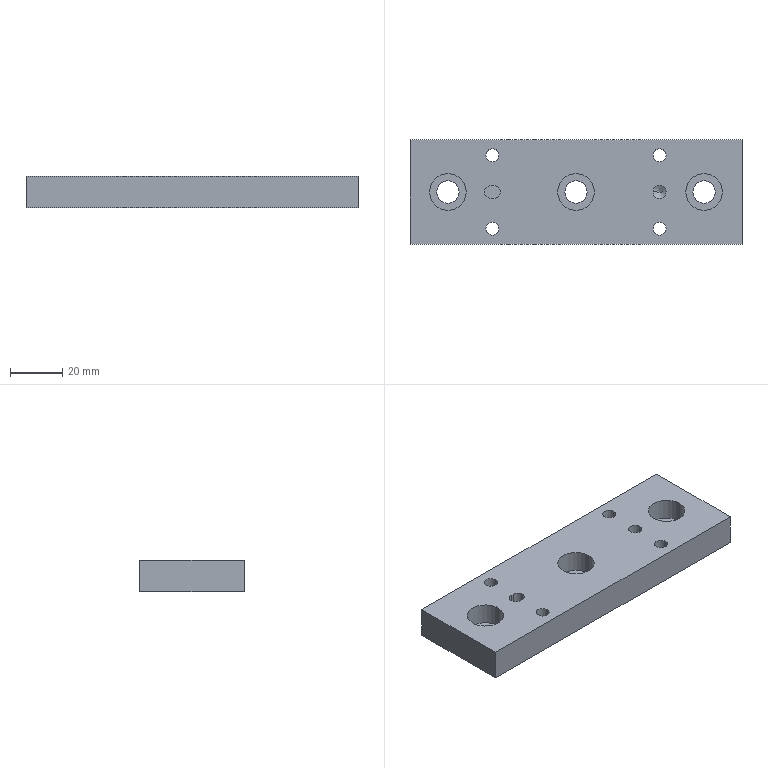Part | STEP file | 1 solid | 42 faces | box 127 x 40 x 12 mm | volume 55019 mm3 | cylinder 27 | plane 13 | cone 2 | commonest cylinder face diameters 5 x13 8.5 x6 14 x6 29.1 x2
STEP:
#1=CARTESIAN_POINT('',(14.55,0.,0.5));
#2=VERTEX_POINT('',#1);
#3=CARTESIAN_POINT('',(-14.55,0.,0.5));
#4=VERTEX_POINT('',#3);
#5=CARTESIAN_POINT('',(0.,0.,0.5));
#6=DIRECTION('',(0.,0.,-1.));
#7=DIRECTION('',(-1.,0.,0.));
#8=AXIS2_PLACEMENT_3D('',#5,#6,#7);
#9=CIRCLE('',#8,14.55);
#10=EDGE_CURVE('',#2,#4,#9,.T.);
#11=ORIENTED_EDGE('',*,*,#10,.F.);
#12=CARTESIAN_POINT('',(14.55,0.,0.));
#13=VERTEX_POINT('',#12);
#14=CARTESIAN_POINT('',(14.55,0.,0.5));
#15=DIRECTION('',(0.,0.,-1.));
#16=VECTOR('',#15,1000.);
#17=LINE('',#14,#16);
#18=EDGE_CURVE('',#2,#13,#17,.T.);
#19=ORIENTED_EDGE('',*,*,#18,.T.);
#20=CARTESIAN_POINT('',(-14.55,0.,0.));
#21=VERTEX_POINT('',#20);
#22=CARTESIAN_POINT('',(0.,0.,0.));
#23=DIRECTION('',(0.,0.,-1.));
#24=DIRECTION('',(-1.,0.,0.));
#25=AXIS2_PLACEMENT_3D('',#22,#23,#24);
#26=CIRCLE('',#25,14.55);
#27=EDGE_CURVE('',#13,#21,#26,.T.);
#28=ORIENTED_EDGE('',*,*,#27,.T.);
#29=CARTESIAN_POINT('',(-14.55,0.,0.5));
#30=DIRECTION('',(0.,0.,-1.));
#31=VECTOR('',#30,1000.);
#32=LINE('',#29,#31);
#33=EDGE_CURVE('',#4,#21,#32,.T.);
#34=ORIENTED_EDGE('',*,*,#33,.F.);
#35=EDGE_LOOP('',(#11,#19,#28,#34));
#36=FACE_OUTER_BOUND('',#35,.T.);
#37=CARTESIAN_POINT('',(0.,0.,0.5));
#38=DIRECTION('',(0.,0.,-1.));
#39=DIRECTION('',(-1.,0.,0.));
#40=AXIS2_PLACEMENT_3D('',#37,#38,#39);
#41=CYLINDRICAL_SURFACE('',#40,14.55);
#42=ADVANCED_FACE('',(#36),#41,.F.);
#43=CARTESIAN_POINT('',(42.,0.,3.7));
#44=VERTEX_POINT('',#43);
#45=CARTESIAN_POINT('',(56.,0.,3.7));
#46=VERTEX_POINT('',#45);
#47=CARTESIAN_POINT('',(49.,0.,3.7));
#48=DIRECTION('',(0.,0.,1.));
#49=DIRECTION('',(1.,0.,0.));
#50=AXIS2_PLACEMENT_3D('',#47,#48,#49);
#51=CIRCLE('',#50,7.);
#52=EDGE_CURVE('',#44,#46,#51,.T.);
#53=ORIENTED_EDGE('',*,*,#52,.F.);
#54=CARTESIAN_POINT('',(42.,0.,12.));
#55=VERTEX_POINT('',#54);
#56=CARTESIAN_POINT('',(42.,0.,12.));
#57=DIRECTION('',(0.,0.,1.));
#58=VECTOR('',#57,1000.);
#59=LINE('',#56,#58);
#60=EDGE_CURVE('',#44,#55,#59,.T.);
#61=ORIENTED_EDGE('',*,*,#60,.T.);
#62=CARTESIAN_POINT('',(56.,0.,12.));
#63=VERTEX_POINT('',#62);
#64=CARTESIAN_POINT('',(49.,0.,12.));
#65=DIRECTION('',(0.,0.,1.));
#66=DIRECTION('',(1.,0.,0.));
#67=AXIS2_PLACEMENT_3D('',#64,#65,#66);
#68=CIRCLE('',#67,7.);
#69=EDGE_CURVE('',#55,#63,#68,.T.);
#70=ORIENTED_EDGE('',*,*,#69,.T.);
#71=CARTESIAN_POINT('',(56.,0.,12.));
#72=DIRECTION('',(0.,0.,1.));
#73=VECTOR('',#72,1000.);
#74=LINE('',#71,#73);
#75=EDGE_CURVE('',#46,#63,#74,.T.);
#76=ORIENTED_EDGE('',*,*,#75,.F.);
#77=EDGE_LOOP('',(#53,#61,#70,#76));
#78=FACE_OUTER_BOUND('',#77,.T.);
#79=CARTESIAN_POINT('',(49.,0.,12.));
#80=DIRECTION('',(0.,0.,1.));
#81=DIRECTION('',(1.,0.,0.));
#82=AXIS2_PLACEMENT_3D('',#79,#80,#81);
#83=CYLINDRICAL_SURFACE('',#82,7.);
#84=ADVANCED_FACE('',(#78),#83,.F.);
#85=CARTESIAN_POINT('',(44.75,0.,0.));
#86=VERTEX_POINT('',#85);
#87=CARTESIAN_POINT('',(53.25,0.,0.));
#88=VERTEX_POINT('',#87);
#89=CARTESIAN_POINT('',(49.,0.,0.));
#90=DIRECTION('',(0.,0.,1.));
#91=DIRECTION('',(1.,0.,0.));
#92=AXIS2_PLACEMENT_3D('',#89,#90,#91);
#93=CIRCLE('',#92,4.25);
#94=EDGE_CURVE('',#86,#88,#93,.T.);
#95=ORIENTED_EDGE('',*,*,#94,.F.);
#96=CARTESIAN_POINT('',(44.75,0.,3.7));
#97=VERTEX_POINT('',#96);
#98=CARTESIAN_POINT('',(44.75,0.,12.));
#99=DIRECTION('',(0.,0.,1.));
#100=VECTOR('',#99,1000.);
#101=LINE('',#98,#100);
#102=EDGE_CURVE('',#86,#97,#101,.T.);
#103=ORIENTED_EDGE('',*,*,#102,.T.);
#104=CARTESIAN_POINT('',(53.25,0.,3.7));
#105=VERTEX_POINT('',#104);
#106=CARTESIAN_POINT('',(49.,0.,3.7));
#107=DIRECTION('',(0.,0.,1.));
#108=DIRECTION('',(1.,0.,0.));
#109=AXIS2_PLACEMENT_3D('',#106,#107,#108);
#110=CIRCLE('',#109,4.25);
#111=EDGE_CURVE('',#97,#105,#110,.T.);
#112=ORIENTED_EDGE('',*,*,#111,.T.);
#113=CARTESIAN_POINT('',(53.25,0.,12.));
#114=DIRECTION('',(0.,0.,1.));
#115=VECTOR('',#114,1000.);
#116=LINE('',#113,#115);
#117=EDGE_CURVE('',#88,#105,#116,.T.);
#118=ORIENTED_EDGE('',*,*,#117,.F.);
#119=EDGE_LOOP('',(#95,#103,#112,#118));
#120=FACE_OUTER_BOUND('',#119,.T.);
#121=CARTESIAN_POINT('',(49.,0.,12.));
#122=DIRECTION('',(0.,0.,1.));
#123=DIRECTION('',(1.,0.,0.));
#124=AXIS2_PLACEMENT_3D('',#121,#122,#123);
#125=CYLINDRICAL_SURFACE('',#124,4.25);
#126=ADVANCED_FACE('',(#120),#125,.F.);
#127=CARTESIAN_POINT('',(-56.,0.,3.7));
#128=VERTEX_POINT('',#127);
#129=CARTESIAN_POINT('',(-42.,0.,3.7));
#130=VERTEX_POINT('',#129);
#131=CARTESIAN_POINT('',(-49.,0.,3.7));
#132=DIRECTION('',(0.,0.,1.));
#133=DIRECTION('',(1.,0.,0.));
#134=AXIS2_PLACEMENT_3D('',#131,#132,#133);
#135=CIRCLE('',#134,7.);
#136=EDGE_CURVE('',#128,#130,#135,.T.);
#137=ORIENTED_EDGE('',*,*,#136,.F.);
#138=CARTESIAN_POINT('',(-56.,0.,12.));
#139=VERTEX_POINT('',#138);
#140=CARTESIAN_POINT('',(-56.,0.,12.));
#141=DIRECTION('',(0.,0.,1.));
#142=VECTOR('',#141,1000.);
#143=LINE('',#140,#142);
#144=EDGE_CURVE('',#128,#139,#143,.T.);
#145=ORIENTED_EDGE('',*,*,#144,.T.);
#146=CARTESIAN_POINT('',(-42.,0.,12.));
#147=VERTEX_POINT('',#146);
#148=CARTESIAN_POINT('',(-49.,0.,12.));
#149=DIRECTION('',(0.,0.,1.));
#150=DIRECTION('',(1.,0.,0.));
#151=AXIS2_PLACEMENT_3D('',#148,#149,#150);
#152=CIRCLE('',#151,7.);
#153=EDGE_CURVE('',#139,#147,#152,.T.);
#154=ORIENTED_EDGE('',*,*,#153,.T.);
#155=CARTESIAN_POINT('',(-42.,0.,12.));
#156=DIRECTION('',(0.,0.,1.));
#157=VECTOR('',#156,1000.);
#158=LINE('',#155,#157);
#159=EDGE_CURVE('',#130,#147,#158,.T.);
#160=ORIENTED_EDGE('',*,*,#159,.F.);
#161=EDGE_LOOP('',(#137,#145,#154,#160));
#162=FACE_OUTER_BOUND('',#161,.T.);
#163=CARTESIAN_POINT('',(-49.,0.,12.));
#164=DIRECTION('',(0.,0.,1.));
#165=DIRECTION('',(1.,0.,0.));
#166=AXIS2_PLACEMENT_3D('',#163,#164,#165);
#167=CYLINDRICAL_SURFACE('',#166,7.);
#168=ADVANCED_FACE('',(#162),#167,.F.);
#169=CARTESIAN_POINT('',(-53.25,0.,0.));
#170=VERTEX_POINT('',#169);
#171=CARTESIAN_POINT('',(-44.75,0.,0.));
#172=VERTEX_POINT('',#171);
#173=CARTESIAN_POINT('',(-49.,0.,0.));
#174=DIRECTION('',(0.,0.,1.));
#175=DIRECTION('',(1.,0.,0.));
#176=AXIS2_PLACEMENT_3D('',#173,#174,#175);
#177=CIRCLE('',#176,4.25);
#178=EDGE_CURVE('',#170,#172,#177,.T.);
#179=ORIENTED_EDGE('',*,*,#178,.F.);
#180=CARTESIAN_POINT('',(-53.25,0.,3.7));
#181=VERTEX_POINT('',#180);
#182=CARTESIAN_POINT('',(-53.25,0.,12.));
#183=DIRECTION('',(0.,0.,1.));
#184=VECTOR('',#183,1000.);
#185=LINE('',#182,#184);
#186=EDGE_CURVE('',#170,#181,#185,.T.);
#187=ORIENTED_EDGE('',*,*,#186,.T.);
#188=CARTESIAN_POINT('',(-44.75,0.,3.7));
#189=VERTEX_POINT('',#188);
#190=CARTESIAN_POINT('',(-49.,0.,3.7));
#191=DIRECTION('',(0.,0.,1.));
#192=DIRECTION('',(1.,0.,0.));
#193=AXIS2_PLACEMENT_3D('',#190,#191,#192);
#194=CIRCLE('',#193,4.25);
#195=EDGE_CURVE('',#181,#189,#194,.T.);
#196=ORIENTED_EDGE('',*,*,#195,.T.);
#197=CARTESIAN_POINT('',(-44.75,0.,12.));
#198=DIRECTION('',(0.,0.,1.));
#199=VECTOR('',#198,1000.);
#200=LINE('',#197,#199);
#201=EDGE_CURVE('',#172,#189,#200,.T.);
#202=ORIENTED_EDGE('',*,*,#201,.F.);
#203=EDGE_LOOP('',(#179,#187,#196,#202));
#204=FACE_OUTER_BOUND('',#203,.T.);
#205=CARTESIAN_POINT('',(-49.,0.,12.));
#206=DIRECTION('',(0.,0.,1.));
#207=DIRECTION('',(1.,0.,0.));
#208=AXIS2_PLACEMENT_3D('',#205,#206,#207);
#209=CYLINDRICAL_SURFACE('',#208,4.25);
#210=ADVANCED_FACE('',(#204),#209,.F.);
#211=CARTESIAN_POINT('',(29.5,14.,0.));
#212=VERTEX_POINT('',#211);
#213=CARTESIAN_POINT('',(34.5,14.,0.));
#214=VERTEX_POINT('',#213);
#215=CARTESIAN_POINT('',(32.,14.,0.));
#216=DIRECTION('',(0.,0.,1.));
#217=DIRECTION('',(1.,0.,0.));
#218=AXIS2_PLACEMENT_3D('',#215,#216,#217);
#219=CIRCLE('',#218,2.5);
#220=EDGE_CURVE('',#212,#214,#219,.T.);
#221=ORIENTED_EDGE('',*,*,#220,.F.);
#222=CARTESIAN_POINT('',(29.5,14.,12.));
#223=VERTEX_POINT('',#222);
#224=CARTESIAN_POINT('',(29.5,14.,12.));
#225=DIRECTION('',(0.,0.,1.));
#226=VECTOR('',#225,1000.);
#227=LINE('',#224,#226);
#228=EDGE_CURVE('',#212,#223,#227,.T.);
#229=ORIENTED_EDGE('',*,*,#228,.T.);
#230=CARTESIAN_POINT('',(34.5,14.,12.));
#231=VERTEX_POINT('',#230);
#232=CARTESIAN_POINT('',(32.,14.,12.));
#233=DIRECTION('',(0.,0.,1.));
#234=DIRECTION('',(1.,0.,0.));
#235=AXIS2_PLACEMENT_3D('',#232,#233,#234);
#236=CIRCLE('',#235,2.5);
#237=EDGE_CURVE('',#223,#231,#236,.T.);
#238=ORIENTED_EDGE('',*,*,#237,.T.);
#239=CARTESIAN_POINT('',(34.5,14.,12.));
#240=DIRECTION('',(0.,0.,1.));
#241=VECTOR('',#240,1000.);
#242=LINE('',#239,#241);
#243=EDGE_CURVE('',#214,#231,#242,.T.);
#244=ORIENTED_EDGE('',*,*,#243,.F.);
#245=EDGE_LOOP('',(#221,#229,#238,#244));
#246=FACE_OUTER_BOUND('',#245,.T.);
#247=CARTESIAN_POINT('',(32.,14.,12.));
#248=DIRECTION('',(0.,0.,1.));
#249=DIRECTION('',(1.,0.,0.));
#250=AXIS2_PLACEMENT_3D('',#247,#248,#249);
#251=CYLINDRICAL_SURFACE('',#250,2.5);
#252=ADVANCED_FACE('',(#246),#251,.F.);
#253=CARTESIAN_POINT('',(29.5,-14.,0.));
#254=VERTEX_POINT('',#253);
#255=CARTESIAN_POINT('',(34.5,-14.,0.));
#256=VERTEX_POINT('',#255);
#257=CARTESIAN_POINT('',(32.,-14.,0.));
#258=DIRECTION('',(0.,0.,1.));
#259=DIRECTION('',(1.,0.,0.));
#260=AXIS2_PLACEMENT_3D('',#257,#258,#259);
#261=CIRCLE('',#260,2.5);
#262=EDGE_CURVE('',#254,#256,#261,.T.);
#263=ORIENTED_EDGE('',*,*,#262,.F.);
#264=CARTESIAN_POINT('',(29.5,-14.,12.));
#265=VERTEX_POINT('',#264);
#266=CARTESIAN_POINT('',(29.5,-14.,12.));
#267=DIRECTION('',(0.,0.,1.));
#268=VECTOR('',#267,1000.);
#269=LINE('',#266,#268);
#270=EDGE_CURVE('',#254,#265,#269,.T.);
#271=ORIENTED_EDGE('',*,*,#270,.T.);
#272=CARTESIAN_POINT('',(34.5,-14.,12.));
#273=VERTEX_POINT('',#272);
#274=CARTESIAN_POINT('',(32.,-14.,12.));
#275=DIRECTION('',(0.,0.,1.));
#276=DIRECTION('',(1.,0.,0.));
#277=AXIS2_PLACEMENT_3D('',#274,#275,#276);
#278=CIRCLE('',#277,2.5);
#279=EDGE_CURVE('',#265,#273,#278,.T.);
#280=ORIENTED_EDGE('',*,*,#279,.T.);
#281=CARTESIAN_POINT('',(34.5,-14.,12.));
#282=DIRECTION('',(0.,0.,1.));
#283=VECTOR('',#282,1000.);
#284=LINE('',#281,#283);
#285=EDGE_CURVE('',#256,#273,#284,.T.);
#286=ORIENTED_EDGE('',*,*,#285,.F.);
#287=EDGE_LOOP('',(#263,#271,#280,#286));
#288=FACE_OUTER_BOUND('',#287,.T.);
#289=CARTESIAN_POINT('',(32.,-14.,12.));
#290=DIRECTION('',(0.,0.,1.));
#291=DIRECTION('',(1.,0.,0.));
#292=AXIS2_PLACEMENT_3D('',#289,#290,#291);
#293=CYLINDRICAL_SURFACE('',#292,2.5);
#294=ADVANCED_FACE('',(#288),#293,.F.);
#295=CARTESIAN_POINT('',(-34.5,-14.,0.));
#296=VERTEX_POINT('',#295);
#297=CARTESIAN_POINT('',(-29.5,-14.,0.));
#298=VERTEX_POINT('',#297);
#299=CARTESIAN_POINT('',(-32.,-14.,0.));
#300=DIRECTION('',(0.,0.,1.));
#301=DIRECTION('',(1.,0.,0.));
#302=AXIS2_PLACEMENT_3D('',#299,#300,#301);
#303=CIRCLE('',#302,2.5);
#304=EDGE_CURVE('',#296,#298,#303,.T.);
#305=ORIENTED_EDGE('',*,*,#304,.F.);
#306=CARTESIAN_POINT('',(-34.5,-14.,12.));
#307=VERTEX_POINT('',#306);
#308=CARTESIAN_POINT('',(-34.5,-14.,12.));
#309=DIRECTION('',(0.,0.,1.));
#310=VECTOR('',#309,1000.);
#311=LINE('',#308,#310);
#312=EDGE_CURVE('',#296,#307,#311,.T.);
#313=ORIENTED_EDGE('',*,*,#312,.T.);
#314=CARTESIAN_POINT('',(-29.5,-14.,12.));
#315=VERTEX_POINT('',#314);
#316=CARTESIAN_POINT('',(-32.,-14.,12.));
#317=DIRECTION('',(0.,0.,1.));
#318=DIRECTION('',(1.,0.,0.));
#319=AXIS2_PLACEMENT_3D('',#316,#317,#318);
#320=CIRCLE('',#319,2.5);
#321=EDGE_CURVE('',#307,#315,#320,.T.);
#322=ORIENTED_EDGE('',*,*,#321,.T.);
#323=CARTESIAN_POINT('',(-29.5,-14.,12.));
#324=DIRECTION('',(0.,0.,1.));
#325=VECTOR('',#324,1000.);
#326=LINE('',#323,#325);
#327=EDGE_CURVE('',#298,#315,#326,.T.);
#328=ORIENTED_EDGE('',*,*,#327,.F.);
#329=EDGE_LOOP('',(#305,#313,#322,#328));
#330=FACE_OUTER_BOUND('',#329,.T.);
#331=CARTESIAN_POINT('',(-32.,-14.,12.));
#332=DIRECTION('',(0.,0.,1.));
#333=DIRECTION('',(1.,0.,0.));
#334=AXIS2_PLACEMENT_3D('',#331,#332,#333);
#335=CYLINDRICAL_SURFACE('',#334,2.5);
#336=ADVANCED_FACE('',(#330),#335,.F.);
#337=CARTESIAN_POINT('',(-34.5,14.,0.));
#338=VERTEX_POINT('',#337);
#339=CARTESIAN_POINT('',(-29.5,14.,0.));
#340=VERTEX_POINT('',#339);
#341=CARTESIAN_POINT('',(-32.,14.,0.));
#342=DIRECTION('',(0.,0.,1.));
#343=DIRECTION('',(1.,0.,0.));
#344=AXIS2_PLACEMENT_3D('',#341,#342,#343);
#345=CIRCLE('',#344,2.5);
#346=EDGE_CURVE('',#338,#340,#345,.T.);
#347=ORIENTED_EDGE('',*,*,#346,.F.);
#348=CARTESIAN_POINT('',(-34.5,14.,12.));
#349=VERTEX_POINT('',#348);
#350=CARTESIAN_POINT('',(-34.5,14.,12.));
#351=DIRECTION('',(0.,0.,1.));
#352=VECTOR('',#351,1000.);
#353=LINE('',#350,#352);
#354=EDGE_CURVE('',#338,#349,#353,.T.);
#355=ORIENTED_EDGE('',*,*,#354,.T.);
#356=CARTESIAN_POINT('',(-29.5,14.,12.));
#357=VERTEX_POINT('',#356);
#358=CARTESIAN_POINT('',(-32.,14.,12.));
#359=DIRECTION('',(0.,0.,1.));
#360=DIRECTION('',(1.,0.,0.));
#361=AXIS2_PLACEMENT_3D('',#358,#359,#360);
#362=CIRCLE('',#361,2.5);
#363=EDGE_CURVE('',#349,#357,#362,.T.);
#364=ORIENTED_EDGE('',*,*,#363,.T.);
#365=CARTESIAN_POINT('',(-29.5,14.,12.));
#366=DIRECTION('',(0.,0.,1.));
#367=VECTOR('',#366,1000.);
#368=LINE('',#365,#367);
#369=EDGE_CURVE('',#340,#357,#368,.T.);
#370=ORIENTED_EDGE('',*,*,#369,.F.);
#371=EDGE_LOOP('',(#347,#355,#364,#370));
#372=FACE_OUTER_BOUND('',#371,.T.);
#373=CARTESIAN_POINT('',(-32.,14.,12.));
#374=DIRECTION('',(0.,0.,1.));
#375=DIRECTION('',(1.,0.,0.));
#376=AXIS2_PLACEMENT_3D('',#373,#374,#375);
#377=CYLINDRICAL_SURFACE('',#376,2.5);
#378=ADVANCED_FACE('',(#372),#377,.F.);
#379=CARTESIAN_POINT('',(-7.,0.,3.7));
#380=VERTEX_POINT('',#379);
#381=CARTESIAN_POINT('',(7.,0.,3.7));
#382=VERTEX_POINT('',#381);
#383=CARTESIAN_POINT('',(0.,0.,3.7));
#384=DIRECTION('',(0.,0.,1.));
#385=DIRECTION('',(1.,0.,0.));
#386=AXIS2_PLACEMENT_3D('',#383,#384,#385);
#387=CIRCLE('',#386,7.);
#388=EDGE_CURVE('',#380,#382,#387,.T.);
#389=ORIENTED_EDGE('',*,*,#388,.F.);
#390=CARTESIAN_POINT('',(-7.,0.,12.));
#391=VERTEX_POINT('',#390);
#392=CARTESIAN_POINT('',(-7.,0.,12.));
#393=DIRECTION('',(0.,0.,1.));
#394=VECTOR('',#393,1000.);
#395=LINE('',#392,#394);
#396=EDGE_CURVE('',#380,#391,#395,.T.);
#397=ORIENTED_EDGE('',*,*,#396,.T.);
#398=CARTESIAN_POINT('',(7.,0.,12.));
#399=VERTEX_POINT('',#398);
#400=CARTESIAN_POINT('',(0.,0.,12.));
#401=DIRECTION('',(0.,0.,1.));
#402=DIRECTION('',(1.,0.,0.));
#403=AXIS2_PLACEMENT_3D('',#400,#401,#402);
#404=CIRCLE('',#403,7.);
#405=EDGE_CURVE('',#391,#399,#404,.T.);
#406=ORIENTED_EDGE('',*,*,#405,.T.);
#407=CARTESIAN_POINT('',(7.,0.,12.));
#408=DIRECTION('',(0.,0.,1.));
#409=VECTOR('',#408,1000.);
#410=LINE('',#407,#409);
#411=EDGE_CURVE('',#382,#399,#410,.T.);
#412=ORIENTED_EDGE('',*,*,#411,.F.);
#413=EDGE_LOOP('',(#389,#397,#406,#412));
#414=FACE_OUTER_BOUND('',#413,.T.);
#415=CARTESIAN_POINT('',(0.,0.,12.));
#416=DIRECTION('',(0.,0.,1.));
#417=DIRECTION('',(1.,0.,0.));
#418=AXIS2_PLACEMENT_3D('',#415,#416,#417);
#419=CYLINDRICAL_SURFACE('',#418,7.);
#420=ADVANCED_FACE('',(#414),#419,.F.);
#421=CARTESIAN_POINT('',(-29.,0.,7.));
#422=VERTEX_POINT('',#421);
#423=CARTESIAN_POINT('',(-31.5,2.5,7.));
#424=VERTEX_POINT('',#423);
#425=CARTESIAN_POINT('',(-31.5,0.,7.));
#426=DIRECTION('',(0.,0.,1.));
#427=DIRECTION('',(1.,0.,0.));
#428=AXIS2_PLACEMENT_3D('',#425,#426,#427);
#429=CIRCLE('',#428,2.5);
#430=EDGE_CURVE('',#422,#424,#429,.T.);
#431=ORIENTED_EDGE('',*,*,#430,.F.);
#432=CARTESIAN_POINT('',(-29.,0.,12.));
#433=VERTEX_POINT('',#432);
#434=CARTESIAN_POINT('',(-29.,0.,7.));
#435=DIRECTION('',(0.,0.,1.));
#436=VECTOR('',#435,1000.);
#437=LINE('',#434,#436);
#438=EDGE_CURVE('',#422,#433,#437,.T.);
#439=ORIENTED_EDGE('',*,*,#438,.T.);
#440=CARTESIAN_POINT('',(-31.5,2.5,12.));
#441=VERTEX_POINT('',#440);
#442=CARTESIAN_POINT('',(-31.5,0.,12.));
#443=DIRECTION('',(0.,0.,1.));
#444=DIRECTION('',(1.,0.,0.));
#445=AXIS2_PLACEMENT_3D('',#442,#443,#444);
#446=CIRCLE('',#445,2.5);
#447=EDGE_CURVE('',#433,#441,#446,.T.);
#448=ORIENTED_EDGE('',*,*,#447,.T.);
#449=CARTESIAN_POINT('',(-31.5,2.5,7.));
#450=DIRECTION('',(0.,0.,1.));
#451=VECTOR('',#450,1000.);
#452=LINE('',#449,#451);
#453=EDGE_CURVE('',#424,#441,#452,.T.);
#454=ORIENTED_EDGE('',*,*,#453,.F.);
#455=EDGE_LOOP('',(#431,#439,#448,#454));
#456=FACE_OUTER_BOUND('',#455,.T.);
#457=CARTESIAN_POINT('',(-31.5,0.,7.));
#458=DIRECTION('',(0.,0.,1.));
#459=DIRECTION('',(1.,0.,0.));
#460=AXIS2_PLACEMENT_3D('',#457,#458,#459);
#461=CYLINDRICAL_SURFACE('',#460,2.5);
#462=ADVANCED_FACE('',(#456),#461,.F.);
#463=CARTESIAN_POINT('',(29.5,0.,7.));
#464=VERTEX_POINT('',#463);
#465=CARTESIAN_POINT('',(34.5,0.,7.));
#466=VERTEX_POINT('',#465);
#467=CARTESIAN_POINT('',(32.,0.,7.));
#468=DIRECTION('',(0.,0.,1.));
#469=DIRECTION('',(1.,0.,0.));
#470=AXIS2_PLACEMENT_3D('',#467,#468,#469);
#471=CIRCLE('',#470,2.5);
#472=EDGE_CURVE('',#464,#466,#471,.T.);
#473=ORIENTED_EDGE('',*,*,#472,.F.);
#474=CARTESIAN_POINT('',(29.5,0.,12.));
#475=VERTEX_POINT('',#474);
#476=CARTESIAN_POINT('',(29.5,0.,12.));
#477=DIRECTION('',(0.,0.,1.));
#478=VECTOR('',#477,1000.);
#479=LINE('',#476,#478);
#480=EDGE_CURVE('',#464,#475,#479,.T.);
#481=ORIENTED_EDGE('',*,*,#480,.T.);
#482=CARTESIAN_POINT('',(34.5,0.,12.));
#483=VERTEX_POINT('',#482);
#484=CARTESIAN_POINT('',(32.,0.,12.));
#485=DIRECTION('',(0.,0.,1.));
#486=DIRECTION('',(1.,0.,0.));
#487=AXIS2_PLACEMENT_3D('',#484,#485,#486);
#488=CIRCLE('',#487,2.5);
#489=EDGE_CURVE('',#475,#483,#488,.T.);
#490=ORIENTED_EDGE('',*,*,#489,.T.);
#491=CARTESIAN_POINT('',(34.5,0.,12.));
#492=DIRECTION('',(0.,0.,1.));
#493=VECTOR('',#492,1000.);
#494=LINE('',#491,#493);
#495=EDGE_CURVE('',#466,#483,#494,.T.);
#496=ORIENTED_EDGE('',*,*,#495,.F.);
#497=EDGE_LOOP('',(#473,#481,#490,#496));
#498=FACE_OUTER_BOUND('',#497,.T.);
#499=CARTESIAN_POINT('',(32.,0.,12.));
#500=DIRECTION('',(0.,0.,1.));
#501=DIRECTION('',(1.,0.,0.));
#502=AXIS2_PLACEMENT_3D('',#499,#500,#501);
#503=CYLINDRICAL_SURFACE('',#502,2.5);
#504=ADVANCED_FACE('',(#498),#503,.F.);
#505=CARTESIAN_POINT('',(32.,0.,5.498));
#506=VERTEX_POINT('',#505);
#507=CARTESIAN_POINT('',(34.5,0.,7.));
#508=DIRECTION('',(0.8572,0.,0.515));
#509=VECTOR('',#508,1000.);
#510=LINE('',#507,#509);
#511=EDGE_CURVE('',#506,#466,#510,.T.);
#512=ORIENTED_EDGE('',*,*,#511,.F.);
#513=CARTESIAN_POINT('',(29.5,0.,7.));
#514=DIRECTION('',(-0.8572,0.,0.515));
#515=VECTOR('',#514,1000.);
#516=LINE('',#513,#515);
#517=EDGE_CURVE('',#506,#464,#516,.T.);
#518=ORIENTED_EDGE('',*,*,#517,.T.);
#519=ORIENTED_EDGE('',*,*,#472,.T.);
#520=EDGE_LOOP('',(#512,#518,#519));
#521=FACE_OUTER_BOUND('',#520,.T.);
#522=CARTESIAN_POINT('',(32.,0.,7.));
#523=DIRECTION('',(0.,0.,1.));
#524=DIRECTION('',(1.,0.,0.));
#525=AXIS2_PLACEMENT_3D('',#522,#523,#524);
#526=CONICAL_SURFACE('',#525,2.5,1.03);
#527=ADVANCED_FACE('',(#521),#526,.F.);
#528=CARTESIAN_POINT('',(-4.25,0.,0.5));
#529=VERTEX_POINT('',#528);
#530=CARTESIAN_POINT('',(4.25,0.,0.5));
#531=VERTEX_POINT('',#530);
#532=CARTESIAN_POINT('',(0.,0.,0.5));
#533=DIRECTION('',(0.,0.,1.));
#534=DIRECTION('',(-1.,0.,0.));
#535=AXIS2_PLACEMENT_3D('',#532,#533,#534);
#536=CIRCLE('',#535,4.25);
#537=EDGE_CURVE('',#529,#531,#536,.T.);
#538=ORIENTED_EDGE('',*,*,#537,.F.);
#539=CARTESIAN_POINT('',(-4.25,0.,3.7));
#540=VERTEX_POINT('',#539);
#541=CARTESIAN_POINT('',(-4.25,0.,12.));
#542=DIRECTION('',(0.,0.,1.));
#543=VECTOR('',#542,1000.);
#544=LINE('',#541,#543);
#545=EDGE_CURVE('',#529,#540,#544,.T.);
#546=ORIENTED_EDGE('',*,*,#545,.T.);
#547=CARTESIAN_POINT('',(4.25,0.,3.7));
#548=VERTEX_POINT('',#547);
#549=CARTESIAN_POINT('',(0.,0.,3.7));
#550=DIRECTION('',(0.,0.,1.));
#551=DIRECTION('',(1.,0.,0.));
#552=AXIS2_PLACEMENT_3D('',#549,#550,#551);
#553=CIRCLE('',#552,4.25);
#554=EDGE_CURVE('',#540,#548,#553,.T.);
#555=ORIENTED_EDGE('',*,*,#554,.T.);
#556=CARTESIAN_POINT('',(4.25,0.,12.));
#557=DIRECTION('',(0.,0.,1.));
#558=VECTOR('',#557,1000.);
#559=LINE('',#556,#558);
#560=EDGE_CURVE('',#531,#548,#559,.T.);
#561=ORIENTED_EDGE('',*,*,#560,.F.);
#562=EDGE_LOOP('',(#538,#546,#555,#561));
#563=FACE_OUTER_BOUND('',#562,.T.);
#564=CARTESIAN_POINT('',(0.,0.,12.));
#565=DIRECTION('',(0.,0.,1.));
#566=DIRECTION('',(1.,0.,0.));
#567=AXIS2_PLACEMENT_3D('',#564,#565,#566);
#568=CYLINDRICAL_SURFACE('',#567,4.25);
#569=ADVANCED_FACE('',(#563),#568,.F.);
#570=ORIENTED_EDGE('',*,*,#545,.F.);
#571=CARTESIAN_POINT('',(0.,0.,0.5));
#572=DIRECTION('',(0.,0.,1.));
#573=DIRECTION('',(-1.,0.,0.));
#574=AXIS2_PLACEMENT_3D('',#571,#572,#573);
#575=CIRCLE('',#574,4.25);
#576=EDGE_CURVE('',#531,#529,#575,.T.);
#577=ORIENTED_EDGE('',*,*,#576,.F.);
#578=ORIENTED_EDGE('',*,*,#560,.T.);
#579=CARTESIAN_POINT('',(0.,0.,3.7));
#580=DIRECTION('',(0.,0.,1.));
#581=DIRECTION('',(1.,0.,0.));
#582=AXIS2_PLACEMENT_3D('',#579,#580,#581);
#583=CIRCLE('',#582,4.25);
#584=EDGE_CURVE('',#548,#540,#583,.T.);
#585=ORIENTED_EDGE('',*,*,#584,.T.);
#586=EDGE_LOOP('',(#570,#577,#578,#585));
#587=FACE_OUTER_BOUND('',#586,.T.);
#588=CARTESIAN_POINT('',(0.,0.,12.));
#589=DIRECTION('',(0.,0.,1.));
#590=DIRECTION('',(1.,0.,0.));
#591=AXIS2_PLACEMENT_3D('',#588,#589,#590);
#592=CYLINDRICAL_SURFACE('',#591,4.25);
#593=ADVANCED_FACE('',(#587),#592,.F.);
#594=CARTESIAN_POINT('',(63.5,-20.,0.));
#595=VERTEX_POINT('',#594);
#596=CARTESIAN_POINT('',(63.5,20.,0.));
#597=VERTEX_POINT('',#596);
#598=CARTESIAN_POINT('',(63.5,-20.,0.));
#599=DIRECTION('',(0.,1.,0.));
#600=VECTOR('',#599,1000.);
#601=LINE('',#598,#600);
#602=EDGE_CURVE('',#595,#597,#601,.T.);
#603=ORIENTED_EDGE('',*,*,#602,.T.);
#604=CARTESIAN_POINT('',(63.5,20.,12.));
#605=VERTEX_POINT('',#604);
#606=CARTESIAN_POINT('',(63.5,20.,12.));
#607=DIRECTION('',(0.,0.,-1.));
#608=VECTOR('',#607,1000.);
#609=LINE('',#606,#608);
#610=EDGE_CURVE('',#605,#597,#609,.T.);
#611=ORIENTED_EDGE('',*,*,#610,.F.);
#612=CARTESIAN_POINT('',(63.5,-20.,12.));
#613=VERTEX_POINT('',#612);
#614=CARTESIAN_POINT('',(63.5,-20.,12.));
#615=DIRECTION('',(0.,1.,0.));
#616=VECTOR('',#615,1000.);
#617=LINE('',#614,#616);
#618=EDGE_CURVE('',#613,#605,#617,.T.);
#619=ORIENTED_EDGE('',*,*,#618,.F.);
#620=CARTESIAN_POINT('',(63.5,-20.,12.));
#621=DIRECTION('',(0.,0.,-1.));
#622=VECTOR('',#621,1000.);
#623=LINE('',#620,#622);
#624=EDGE_CURVE('',#613,#595,#623,.T.);
#625=ORIENTED_EDGE('',*,*,#624,.T.);
#626=EDGE_LOOP('',(#603,#611,#619,#625));
#627=FACE_OUTER_BOUND('',#626,.T.);
#628=CARTESIAN_POINT('',(63.5,-20.,12.));
#629=DIRECTION('',(-1.,0.,0.));
#630=DIRECTION('',(0.,0.,1.));
#631=AXIS2_PLACEMENT_3D('',#628,#629,#630);
#632=PLANE('',#631);
#633=ADVANCED_FACE('',(#627),#632,.F.);
#634=CARTESIAN_POINT('',(-63.5,20.,0.));
#635=VERTEX_POINT('',#634);
#636=CARTESIAN_POINT('',(-63.5,20.,0.));
#637=DIRECTION('',(-1.,0.,0.));
#638=VECTOR('',#637,1000.);
#639=LINE('',#636,#638);
#640=EDGE_CURVE('',#597,#635,#639,.T.);
#641=ORIENTED_EDGE('',*,*,#640,.T.);
#642=CARTESIAN_POINT('',(-63.5,20.,12.));
#643=VERTEX_POINT('',#642);
#644=CARTESIAN_POINT('',(-63.5,20.,12.));
#645=DIRECTION('',(0.,0.,-1.));
#646=VECTOR('',#645,1000.);
#647=LINE('',#644,#646);
#648=EDGE_CURVE('',#643,#635,#647,.T.);
#649=ORIENTED_EDGE('',*,*,#648,.F.);
#650=CARTESIAN_POINT('',(-63.5,20.,12.));
#651=DIRECTION('',(-1.,0.,0.));
#652=VECTOR('',#651,1000.);
#653=LINE('',#650,#652);
#654=EDGE_CURVE('',#605,#643,#653,.T.);
#655=ORIENTED_EDGE('',*,*,#654,.F.);
#656=ORIENTED_EDGE('',*,*,#610,.T.);
#657=EDGE_LOOP('',(#641,#649,#655,#656));
#658=FACE_OUTER_BOUND('',#657,.T.);
#659=CARTESIAN_POINT('',(-63.5,20.,12.));
#660=DIRECTION('',(0.,-1.,0.));
#661=DIRECTION('',(0.,0.,-1.));
#662=AXIS2_PLACEMENT_3D('',#659,#660,#661);
#663=PLANE('',#662);
#664=ADVANCED_FACE('',(#658),#663,.F.);
#665=CARTESIAN_POINT('',(-63.5,-20.,0.));
#666=VERTEX_POINT('',#665);
#667=CARTESIAN_POINT('',(-63.5,-20.,0.));
#668=DIRECTION('',(0.,-1.,0.));
#669=VECTOR('',#668,1000.);
#670=LINE('',#667,#669);
#671=EDGE_CURVE('',#635,#666,#670,.T.);
#672=ORIENTED_EDGE('',*,*,#671,.T.);
#673=CARTESIAN_POINT('',(-63.5,-20.,12.));
#674=VERTEX_POINT('',#673);
#675=CARTESIAN_POINT('',(-63.5,-20.,12.));
#676=DIRECTION('',(0.,0.,-1.));
#677=VECTOR('',#676,1000.);
#678=LINE('',#675,#677);
#679=EDGE_CURVE('',#674,#666,#678,.T.);
#680=ORIENTED_EDGE('',*,*,#679,.F.);
#681=CARTESIAN_POINT('',(-63.5,-20.,12.));
#682=DIRECTION('',(0.,-1.,0.));
#683=VECTOR('',#682,1000.);
#684=LINE('',#681,#683);
#685=EDGE_CURVE('',#643,#674,#684,.T.);
#686=ORIENTED_EDGE('',*,*,#685,.F.);
#687=ORIENTED_EDGE('',*,*,#648,.T.);
#688=EDGE_LOOP('',(#672,#680,#686,#687));
#689=FACE_OUTER_BOUND('',#688,.T.);
#690=CARTESIAN_POINT('',(-63.5,-20.,12.));
#691=DIRECTION('',(1.,0.,0.));
#692=DIRECTION('',(0.,1.,0.));
#693=AXIS2_PLACEMENT_3D('',#690,#691,#692);
#694=PLANE('',#693);
#695=ADVANCED_FACE('',(#689),#694,.F.);
#696=CARTESIAN_POINT('',(-63.5,-20.,0.));
#697=DIRECTION('',(1.,0.,0.));
#698=VECTOR('',#697,1000.);
#699=LINE('',#696,#698);
#700=EDGE_CURVE('',#666,#595,#699,.T.);
#701=ORIENTED_EDGE('',*,*,#700,.T.);
#702=ORIENTED_EDGE('',*,*,#624,.F.);
#703=CARTESIAN_POINT('',(-63.5,-20.,12.));
#704=DIRECTION('',(1.,0.,0.));
#705=VECTOR('',#704,1000.);
#706=LINE('',#703,#705);
#707=EDGE_CURVE('',#674,#613,#706,.T.);
#708=ORIENTED_EDGE('',*,*,#707,.F.);
#709=ORIENTED_EDGE('',*,*,#679,.T.);
#710=EDGE_LOOP('',(#701,#702,#708,#709));
#711=FACE_OUTER_BOUND('',#710,.T.);
#712=CARTESIAN_POINT('',(-63.5,-20.,12.));
#713=DIRECTION('',(0.,1.,0.));
#714=DIRECTION('',(1.,0.,0.));
#715=AXIS2_PLACEMENT_3D('',#712,#713,#714);
#716=PLANE('',#715);
#717=ADVANCED_FACE('',(#711),#716,.F.);
#718=ORIENTED_EDGE('',*,*,#618,.T.);
#719=ORIENTED_EDGE('',*,*,#654,.T.);
#720=ORIENTED_EDGE('',*,*,#685,.T.);
#721=ORIENTED_EDGE('',*,*,#707,.T.);
#722=EDGE_LOOP('',(#718,#719,#720,#721));
#723=FACE_OUTER_BOUND('',#722,.T.);
#724=CARTESIAN_POINT('',(49.,0.,12.));
#725=DIRECTION('',(0.,0.,1.));
#726=DIRECTION('',(1.,0.,0.));
#727=AXIS2_PLACEMENT_3D('',#724,#725,#726);
#728=CIRCLE('',#727,7.);
#729=EDGE_CURVE('',#63,#55,#728,.T.);
#730=ORIENTED_EDGE('',*,*,#729,.F.);
#731=ORIENTED_EDGE('',*,*,#69,.F.);
#732=EDGE_LOOP('',(#730,#731));
#733=FACE_BOUND('',#732,.T.);
#734=CARTESIAN_POINT('',(-49.,0.,12.));
#735=DIRECTION('',(0.,0.,1.));
#736=DIRECTION('',(1.,0.,0.));
#737=AXIS2_PLACEMENT_3D('',#734,#735,#736);
#738=CIRCLE('',#737,7.);
#739=EDGE_CURVE('',#147,#139,#738,.T.);
#740=ORIENTED_EDGE('',*,*,#739,.F.);
#741=ORIENTED_EDGE('',*,*,#153,.F.);
#742=EDGE_LOOP('',(#740,#741));
#743=FACE_BOUND('',#742,.T.);
#744=CARTESIAN_POINT('',(32.,14.,12.));
#745=DIRECTION('',(0.,0.,1.));
#746=DIRECTION('',(1.,0.,0.));
#747=AXIS2_PLACEMENT_3D('',#744,#745,#746);
#748=CIRCLE('',#747,2.5);
#749=EDGE_CURVE('',#231,#223,#748,.T.);
#750=ORIENTED_EDGE('',*,*,#749,.F.);
#751=ORIENTED_EDGE('',*,*,#237,.F.);
#752=EDGE_LOOP('',(#750,#751));
#753=FACE_BOUND('',#752,.T.);
#754=CARTESIAN_POINT('',(32.,-14.,12.));
#755=DIRECTION('',(0.,0.,1.));
#756=DIRECTION('',(1.,0.,0.));
#757=AXIS2_PLACEMENT_3D('',#754,#755,#756);
#758=CIRCLE('',#757,2.5);
#759=EDGE_CURVE('',#273,#265,#758,.T.);
#760=ORIENTED_EDGE('',*,*,#759,.F.);
#761=ORIENTED_EDGE('',*,*,#279,.F.);
#762=EDGE_LOOP('',(#760,#761));
#763=FACE_BOUND('',#762,.T.);
#764=CARTESIAN_POINT('',(-32.,-14.,12.));
#765=DIRECTION('',(0.,0.,1.));
#766=DIRECTION('',(1.,0.,0.));
#767=AXIS2_PLACEMENT_3D('',#764,#765,#766);
#768=CIRCLE('',#767,2.5);
#769=EDGE_CURVE('',#315,#307,#768,.T.);
#770=ORIENTED_EDGE('',*,*,#769,.F.);
#771=ORIENTED_EDGE('',*,*,#321,.F.);
#772=EDGE_LOOP('',(#770,#771));
#773=FACE_BOUND('',#772,.T.);
#774=CARTESIAN_POINT('',(-32.,14.,12.));
#775=DIRECTION('',(0.,0.,1.));
#776=DIRECTION('',(1.,0.,0.));
#777=AXIS2_PLACEMENT_3D('',#774,#775,#776);
#778=CIRCLE('',#777,2.5);
#779=EDGE_CURVE('',#357,#349,#778,.T.);
#780=ORIENTED_EDGE('',*,*,#779,.F.);
#781=ORIENTED_EDGE('',*,*,#363,.F.);
#782=EDGE_LOOP('',(#780,#781));
#783=FACE_BOUND('',#782,.T.);
#784=CARTESIAN_POINT('',(0.,0.,12.));
#785=DIRECTION('',(0.,0.,1.));
#786=DIRECTION('',(1.,0.,0.));
#787=AXIS2_PLACEMENT_3D('',#784,#785,#786);
#788=CIRCLE('',#787,7.);
#789=EDGE_CURVE('',#399,#391,#788,.T.);
#790=ORIENTED_EDGE('',*,*,#789,.F.);
#791=ORIENTED_EDGE('',*,*,#405,.F.);
#792=EDGE_LOOP('',(#790,#791));
#793=FACE_BOUND('',#792,.T.);
#794=CARTESIAN_POINT('',(-32.5,-2.5,12.));
#795=VERTEX_POINT('',#794);
#796=CARTESIAN_POINT('',(-31.5,-2.5,12.));
#797=VERTEX_POINT('',#796);
#798=CARTESIAN_POINT('',(-32.5,-2.5,12.));
#799=DIRECTION('',(1.,0.,0.));
#800=VECTOR('',#799,1000.);
#801=LINE('',#798,#800);
#802=EDGE_CURVE('',#795,#797,#801,.T.);
#803=ORIENTED_EDGE('',*,*,#802,.F.);
#804=CARTESIAN_POINT('',(-32.5,2.5,12.));
#805=VERTEX_POINT('',#804);
#806=CARTESIAN_POINT('',(-32.5,0.,12.));
#807=DIRECTION('',(0.,0.,1.));
#808=DIRECTION('',(1.,0.,0.));
#809=AXIS2_PLACEMENT_3D('',#806,#807,#808);
#810=CIRCLE('',#809,2.5);
#811=EDGE_CURVE('',#805,#795,#810,.T.);
#812=ORIENTED_EDGE('',*,*,#811,.F.);
#813=CARTESIAN_POINT('',(-32.5,2.5,12.));
#814=DIRECTION('',(-1.,0.,0.));
#815=VECTOR('',#814,1000.);
#816=LINE('',#813,#815);
#817=EDGE_CURVE('',#441,#805,#816,.T.);
#818=ORIENTED_EDGE('',*,*,#817,.F.);
#819=ORIENTED_EDGE('',*,*,#447,.F.);
#820=CARTESIAN_POINT('',(-31.5,0.,12.));
#821=DIRECTION('',(0.,0.,1.));
#822=DIRECTION('',(1.,0.,0.));
#823=AXIS2_PLACEMENT_3D('',#820,#821,#822);
#824=CIRCLE('',#823,2.5);
#825=EDGE_CURVE('',#797,#433,#824,.T.);
#826=ORIENTED_EDGE('',*,*,#825,.F.);
#827=EDGE_LOOP('',(#803,#812,#818,#819,#826));
#828=FACE_BOUND('',#827,.T.);
#829=CARTESIAN_POINT('',(32.,0.,12.));
#830=DIRECTION('',(0.,0.,1.));
#831=DIRECTION('',(1.,0.,0.));
#832=AXIS2_PLACEMENT_3D('',#829,#830,#831);
#833=CIRCLE('',#832,2.5);
#834=EDGE_CURVE('',#483,#475,#833,.T.);
#835=ORIENTED_EDGE('',*,*,#834,.F.);
#836=ORIENTED_EDGE('',*,*,#489,.F.);
#837=EDGE_LOOP('',(#835,#836));
#838=FACE_BOUND('',#837,.T.);
#839=CARTESIAN_POINT('',(0.,0.,12.));
#840=DIRECTION('',(0.,0.,-1.));
#841=DIRECTION('',(0.,-1.,0.));
#842=AXIS2_PLACEMENT_3D('',#839,#840,#841);
#843=PLANE('',#842);
#844=ADVANCED_FACE('',(#723,#733,#743,#753,#763,#773,#783,#793,#828,#838),#843,.F.);
#845=ORIENTED_EDGE('',*,*,#602,.F.);
#846=ORIENTED_EDGE('',*,*,#700,.F.);
#847=ORIENTED_EDGE('',*,*,#671,.F.);
#848=ORIENTED_EDGE('',*,*,#640,.F.);
#849=EDGE_LOOP('',(#845,#846,#847,#848));
#850=FACE_OUTER_BOUND('',#849,.T.);
#851=CARTESIAN_POINT('',(0.,0.,0.));
#852=DIRECTION('',(0.,0.,-1.));
#853=DIRECTION('',(-1.,0.,0.));
#854=AXIS2_PLACEMENT_3D('',#851,#852,#853);
#855=CIRCLE('',#854,14.55);
#856=EDGE_CURVE('',#21,#13,#855,.T.);
#857=ORIENTED_EDGE('',*,*,#856,.F.);
#858=ORIENTED_EDGE('',*,*,#27,.F.);
#859=EDGE_LOOP('',(#857,#858));
#860=FACE_BOUND('',#859,.T.);
#861=CARTESIAN_POINT('',(49.,0.,0.));
#862=DIRECTION('',(0.,0.,1.));
#863=DIRECTION('',(1.,0.,0.));
#864=AXIS2_PLACEMENT_3D('',#861,#862,#863);
#865=CIRCLE('',#864,4.25);
#866=EDGE_CURVE('',#88,#86,#865,.T.);
#867=ORIENTED_EDGE('',*,*,#866,.T.);
#868=ORIENTED_EDGE('',*,*,#94,.T.);
#869=EDGE_LOOP('',(#867,#868));
#870=FACE_BOUND('',#869,.T.);
#871=CARTESIAN_POINT('',(-49.,0.,0.));
#872=DIRECTION('',(0.,0.,1.));
#873=DIRECTION('',(1.,0.,0.));
#874=AXIS2_PLACEMENT_3D('',#871,#872,#873);
#875=CIRCLE('',#874,4.25);
#876=EDGE_CURVE('',#172,#170,#875,.T.);
#877=ORIENTED_EDGE('',*,*,#876,.T.);
#878=ORIENTED_EDGE('',*,*,#178,.T.);
#879=EDGE_LOOP('',(#877,#878));
#880=FACE_BOUND('',#879,.T.);
#881=CARTESIAN_POINT('',(32.,14.,0.));
#882=DIRECTION('',(0.,0.,1.));
#883=DIRECTION('',(1.,0.,0.));
#884=AXIS2_PLACEMENT_3D('',#881,#882,#883);
#885=CIRCLE('',#884,2.5);
#886=EDGE_CURVE('',#214,#212,#885,.T.);
#887=ORIENTED_EDGE('',*,*,#886,.T.);
#888=ORIENTED_EDGE('',*,*,#220,.T.);
#889=EDGE_LOOP('',(#887,#888));
#890=FACE_BOUND('',#889,.T.);
#891=CARTESIAN_POINT('',(32.,-14.,0.));
#892=DIRECTION('',(0.,0.,1.));
#893=DIRECTION('',(1.,0.,0.));
#894=AXIS2_PLACEMENT_3D('',#891,#892,#893);
#895=CIRCLE('',#894,2.5);
#896=EDGE_CURVE('',#256,#254,#895,.T.);
#897=ORIENTED_EDGE('',*,*,#896,.T.);
#898=ORIENTED_EDGE('',*,*,#262,.T.);
#899=EDGE_LOOP('',(#897,#898));
#900=FACE_BOUND('',#899,.T.);
#901=CARTESIAN_POINT('',(-32.,-14.,0.));
#902=DIRECTION('',(0.,0.,1.));
#903=DIRECTION('',(1.,0.,0.));
#904=AXIS2_PLACEMENT_3D('',#901,#902,#903);
#905=CIRCLE('',#904,2.5);
#906=EDGE_CURVE('',#298,#296,#905,.T.);
#907=ORIENTED_EDGE('',*,*,#906,.T.);
#908=ORIENTED_EDGE('',*,*,#304,.T.);
#909=EDGE_LOOP('',(#907,#908));
#910=FACE_BOUND('',#909,.T.);
#911=CARTESIAN_POINT('',(-32.,14.,0.));
#912=DIRECTION('',(0.,0.,1.));
#913=DIRECTION('',(1.,0.,0.));
#914=AXIS2_PLACEMENT_3D('',#911,#912,#913);
#915=CIRCLE('',#914,2.5);
#916=EDGE_CURVE('',#340,#338,#915,.T.);
#917=ORIENTED_EDGE('',*,*,#916,.T.);
#918=ORIENTED_EDGE('',*,*,#346,.T.);
#919=EDGE_LOOP('',(#917,#918));
#920=FACE_BOUND('',#919,.T.);
#921=CARTESIAN_POINT('',(0.,0.,0.));
#922=DIRECTION('',(0.,0.,-1.));
#923=DIRECTION('',(0.,-1.,0.));
#924=AXIS2_PLACEMENT_3D('',#921,#922,#923);
#925=PLANE('',#924);
#926=ADVANCED_FACE('',(#850,#860,#870,#880,#890,#900,#910,#920),#925,.T.);
#927=ORIENTED_EDGE('',*,*,#517,.F.);
#928=ORIENTED_EDGE('',*,*,#511,.T.);
#929=CARTESIAN_POINT('',(32.,0.,7.));
#930=DIRECTION('',(0.,0.,1.));
#931=DIRECTION('',(1.,0.,0.));
#932=AXIS2_PLACEMENT_3D('',#929,#930,#931);
#933=CIRCLE('',#932,2.5);
#934=EDGE_CURVE('',#466,#464,#933,.T.);
#935=ORIENTED_EDGE('',*,*,#934,.T.);
#936=EDGE_LOOP('',(#927,#928,#935));
#937=FACE_OUTER_BOUND('',#936,.T.);
#938=CARTESIAN_POINT('',(32.,0.,7.));
#939=DIRECTION('',(0.,0.,1.));
#940=DIRECTION('',(1.,0.,0.));
#941=AXIS2_PLACEMENT_3D('',#938,#939,#940);
#942=CONICAL_SURFACE('',#941,2.5,1.03);
#943=ADVANCED_FACE('',(#937),#942,.F.);
#944=ORIENTED_EDGE('',*,*,#480,.F.);
#945=ORIENTED_EDGE('',*,*,#934,.F.);
#946=ORIENTED_EDGE('',*,*,#495,.T.);
#947=ORIENTED_EDGE('',*,*,#834,.T.);
#948=EDGE_LOOP('',(#944,#945,#946,#947));
#949=FACE_OUTER_BOUND('',#948,.T.);
#950=CARTESIAN_POINT('',(32.,0.,12.));
#951=DIRECTION('',(0.,0.,1.));
#952=DIRECTION('',(1.,0.,0.));
#953=AXIS2_PLACEMENT_3D('',#950,#951,#952);
#954=CYLINDRICAL_SURFACE('',#953,2.5);
#955=ADVANCED_FACE('',(#949),#954,.F.);
#956=ORIENTED_EDGE('',*,*,#811,.T.);
#957=CARTESIAN_POINT('',(-32.5,-2.5,7.));
#958=VERTEX_POINT('',#957);
#959=CARTESIAN_POINT('',(-32.5,-2.5,7.));
#960=DIRECTION('',(0.,0.,1.));
#961=VECTOR('',#960,1000.);
#962=LINE('',#959,#961);
#963=EDGE_CURVE('',#958,#795,#962,.T.);
#964=ORIENTED_EDGE('',*,*,#963,.F.);
#965=CARTESIAN_POINT('',(-32.5,2.5,7.));
#966=VERTEX_POINT('',#965);
#967=CARTESIAN_POINT('',(-32.5,0.,7.));
#968=DIRECTION('',(0.,0.,1.));
#969=DIRECTION('',(1.,0.,0.));
#970=AXIS2_PLACEMENT_3D('',#967,#968,#969);
#971=CIRCLE('',#970,2.5);
#972=EDGE_CURVE('',#966,#958,#971,.T.);
#973=ORIENTED_EDGE('',*,*,#972,.F.);
#974=CARTESIAN_POINT('',(-32.5,2.5,7.));
#975=DIRECTION('',(0.,0.,1.));
#976=VECTOR('',#975,1000.);
#977=LINE('',#974,#976);
#978=EDGE_CURVE('',#966,#805,#977,.T.);
#979=ORIENTED_EDGE('',*,*,#978,.T.);
#980=EDGE_LOOP('',(#956,#964,#973,#979));
#981=FACE_OUTER_BOUND('',#980,.T.);
#982=CARTESIAN_POINT('',(-32.5,0.,7.));
#983=DIRECTION('',(0.,0.,1.));
#984=DIRECTION('',(1.,0.,0.));
#985=AXIS2_PLACEMENT_3D('',#982,#983,#984);
#986=CYLINDRICAL_SURFACE('',#985,2.5);
#987=ADVANCED_FACE('',(#981),#986,.F.);
#988=ORIENTED_EDGE('',*,*,#817,.T.);
#989=ORIENTED_EDGE('',*,*,#978,.F.);
#990=CARTESIAN_POINT('',(-32.5,2.5,7.));
#991=DIRECTION('',(-1.,0.,0.));
#992=VECTOR('',#991,1000.);
#993=LINE('',#990,#992);
#994=EDGE_CURVE('',#424,#966,#993,.T.);
#995=ORIENTED_EDGE('',*,*,#994,.F.);
#996=ORIENTED_EDGE('',*,*,#453,.T.);
#997=EDGE_LOOP('',(#988,#989,#995,#996));
#998=FACE_OUTER_BOUND('',#997,.T.);
#999=CARTESIAN_POINT('',(-32.5,2.5,7.));
#1000=DIRECTION('',(0.,1.,0.));
#1001=DIRECTION('',(1.,0.,0.));
#1002=AXIS2_PLACEMENT_3D('',#999,#1000,#1001);
#1003=PLANE('',#1002);
#1004=ADVANCED_FACE('',(#998),#1003,.F.);
#1005=ORIENTED_EDGE('',*,*,#438,.F.);
#1006=CARTESIAN_POINT('',(-31.5,-2.5,7.));
#1007=VERTEX_POINT('',#1006);
#1008=CARTESIAN_POINT('',(-31.5,0.,7.));
#1009=DIRECTION('',(0.,0.,1.));
#1010=DIRECTION('',(1.,0.,0.));
#1011=AXIS2_PLACEMENT_3D('',#1008,#1009,#1010);
#1012=CIRCLE('',#1011,2.5);
#1013=EDGE_CURVE('',#1007,#422,#1012,.T.);
#1014=ORIENTED_EDGE('',*,*,#1013,.F.);
#1015=CARTESIAN_POINT('',(-31.5,-2.5,7.));
#1016=DIRECTION('',(0.,0.,1.));
#1017=VECTOR('',#1016,1000.);
#1018=LINE('',#1015,#1017);
#1019=EDGE_CURVE('',#1007,#797,#1018,.T.);
#1020=ORIENTED_EDGE('',*,*,#1019,.T.);
#1021=ORIENTED_EDGE('',*,*,#825,.T.);
#1022=EDGE_LOOP('',(#1005,#1014,#1020,#1021));
#1023=FACE_OUTER_BOUND('',#1022,.T.);
#1024=CARTESIAN_POINT('',(-31.5,0.,7.));
#1025=DIRECTION('',(0.,0.,1.));
#1026=DIRECTION('',(1.,0.,0.));
#1027=AXIS2_PLACEMENT_3D('',#1024,#1025,#1026);
#1028=CYLINDRICAL_SURFACE('',#1027,2.5);
#1029=ADVANCED_FACE('',(#1023),#1028,.F.);
#1030=ORIENTED_EDGE('',*,*,#802,.T.);
#1031=ORIENTED_EDGE('',*,*,#1019,.F.);
#1032=CARTESIAN_POINT('',(-32.5,-2.5,7.));
#1033=DIRECTION('',(1.,0.,0.));
#1034=VECTOR('',#1033,1000.);
#1035=LINE('',#1032,#1034);
#1036=EDGE_CURVE('',#958,#1007,#1035,.T.);
#1037=ORIENTED_EDGE('',*,*,#1036,.F.);
#1038=ORIENTED_EDGE('',*,*,#963,.T.);
#1039=EDGE_LOOP('',(#1030,#1031,#1037,#1038));
#1040=FACE_OUTER_BOUND('',#1039,.T.);
#1041=CARTESIAN_POINT('',(-32.5,-2.5,7.));
#1042=DIRECTION('',(0.,-1.,0.));
#1043=DIRECTION('',(0.,0.,-1.));
#1044=AXIS2_PLACEMENT_3D('',#1041,#1042,#1043);
#1045=PLANE('',#1044);
#1046=ADVANCED_FACE('',(#1040),#1045,.F.);
#1047=ORIENTED_EDGE('',*,*,#972,.T.);
#1048=ORIENTED_EDGE('',*,*,#1036,.T.);
#1049=ORIENTED_EDGE('',*,*,#1013,.T.);
#1050=ORIENTED_EDGE('',*,*,#430,.T.);
#1051=ORIENTED_EDGE('',*,*,#994,.T.);
#1052=EDGE_LOOP('',(#1047,#1048,#1049,#1050,#1051));
#1053=FACE_OUTER_BOUND('',#1052,.T.);
#1054=CARTESIAN_POINT('',(-32.5,0.,7.));
#1055=DIRECTION('',(0.,0.,1.));
#1056=DIRECTION('',(1.,0.,0.));
#1057=AXIS2_PLACEMENT_3D('',#1054,#1055,#1056);
#1058=PLANE('',#1057);
#1059=ADVANCED_FACE('',(#1053),#1058,.T.);
#1060=CARTESIAN_POINT('',(0.,0.,3.7));
#1061=DIRECTION('',(0.,0.,1.));
#1062=DIRECTION('',(1.,0.,0.));
#1063=AXIS2_PLACEMENT_3D('',#1060,#1061,#1062);
#1064=CIRCLE('',#1063,7.);
#1065=EDGE_CURVE('',#382,#380,#1064,.T.);
#1066=ORIENTED_EDGE('',*,*,#1065,.T.);
#1067=ORIENTED_EDGE('',*,*,#388,.T.);
#1068=EDGE_LOOP('',(#1066,#1067));
#1069=FACE_OUTER_BOUND('',#1068,.T.);
#1070=ORIENTED_EDGE('',*,*,#584,.F.);
#1071=ORIENTED_EDGE('',*,*,#554,.F.);
#1072=EDGE_LOOP('',(#1070,#1071));
#1073=FACE_BOUND('',#1072,.T.);
#1074=CARTESIAN_POINT('',(4.25,0.,3.7));
#1075=DIRECTION('',(0.,0.,-1.));
#1076=DIRECTION('',(0.,-1.,0.));
#1077=AXIS2_PLACEMENT_3D('',#1074,#1075,#1076);
#1078=PLANE('',#1077);
#1079=ADVANCED_FACE('',(#1069,#1073),#1078,.F.);
#1080=ORIENTED_EDGE('',*,*,#396,.F.);
#1081=ORIENTED_EDGE('',*,*,#1065,.F.);
#1082=ORIENTED_EDGE('',*,*,#411,.T.);
#1083=ORIENTED_EDGE('',*,*,#789,.T.);
#1084=EDGE_LOOP('',(#1080,#1081,#1082,#1083));
#1085=FACE_OUTER_BOUND('',#1084,.T.);
#1086=CARTESIAN_POINT('',(0.,0.,12.));
#1087=DIRECTION('',(0.,0.,1.));
#1088=DIRECTION('',(1.,0.,0.));
#1089=AXIS2_PLACEMENT_3D('',#1086,#1087,#1088);
#1090=CYLINDRICAL_SURFACE('',#1089,7.);
#1091=ADVANCED_FACE('',(#1085),#1090,.F.);
#1092=ORIENTED_EDGE('',*,*,#354,.F.);
#1093=ORIENTED_EDGE('',*,*,#916,.F.);
#1094=ORIENTED_EDGE('',*,*,#369,.T.);
#1095=ORIENTED_EDGE('',*,*,#779,.T.);
#1096=EDGE_LOOP('',(#1092,#1093,#1094,#1095));
#1097=FACE_OUTER_BOUND('',#1096,.T.);
#1098=CARTESIAN_POINT('',(-32.,14.,12.));
#1099=DIRECTION('',(0.,0.,1.));
#1100=DIRECTION('',(1.,0.,0.));
#1101=AXIS2_PLACEMENT_3D('',#1098,#1099,#1100);
#1102=CYLINDRICAL_SURFACE('',#1101,2.5);
#1103=ADVANCED_FACE('',(#1097),#1102,.F.);
#1104=ORIENTED_EDGE('',*,*,#312,.F.);
#1105=ORIENTED_EDGE('',*,*,#906,.F.);
#1106=ORIENTED_EDGE('',*,*,#327,.T.);
#1107=ORIENTED_EDGE('',*,*,#769,.T.);
#1108=EDGE_LOOP('',(#1104,#1105,#1106,#1107));
#1109=FACE_OUTER_BOUND('',#1108,.T.);
#1110=CARTESIAN_POINT('',(-32.,-14.,12.));
#1111=DIRECTION('',(0.,0.,1.));
#1112=DIRECTION('',(1.,0.,0.));
#1113=AXIS2_PLACEMENT_3D('',#1110,#1111,#1112);
#1114=CYLINDRICAL_SURFACE('',#1113,2.5);
#1115=ADVANCED_FACE('',(#1109),#1114,.F.);
#1116=ORIENTED_EDGE('',*,*,#270,.F.);
#1117=ORIENTED_EDGE('',*,*,#896,.F.);
#1118=ORIENTED_EDGE('',*,*,#285,.T.);
#1119=ORIENTED_EDGE('',*,*,#759,.T.);
#1120=EDGE_LOOP('',(#1116,#1117,#1118,#1119));
#1121=FACE_OUTER_BOUND('',#1120,.T.);
#1122=CARTESIAN_POINT('',(32.,-14.,12.));
#1123=DIRECTION('',(0.,0.,1.));
#1124=DIRECTION('',(1.,0.,0.));
#1125=AXIS2_PLACEMENT_3D('',#1122,#1123,#1124);
#1126=CYLINDRICAL_SURFACE('',#1125,2.5);
#1127=ADVANCED_FACE('',(#1121),#1126,.F.);
#1128=ORIENTED_EDGE('',*,*,#228,.F.);
#1129=ORIENTED_EDGE('',*,*,#886,.F.);
#1130=ORIENTED_EDGE('',*,*,#243,.T.);
#1131=ORIENTED_EDGE('',*,*,#749,.T.);
#1132=EDGE_LOOP('',(#1128,#1129,#1130,#1131));
#1133=FACE_OUTER_BOUND('',#1132,.T.);
#1134=CARTESIAN_POINT('',(32.,14.,12.));
#1135=DIRECTION('',(0.,0.,1.));
#1136=DIRECTION('',(1.,0.,0.));
#1137=AXIS2_PLACEMENT_3D('',#1134,#1135,#1136);
#1138=CYLINDRICAL_SURFACE('',#1137,2.5);
#1139=ADVANCED_FACE('',(#1133),#1138,.F.);
#1140=ORIENTED_EDGE('',*,*,#186,.F.);
#1141=ORIENTED_EDGE('',*,*,#876,.F.);
#1142=ORIENTED_EDGE('',*,*,#201,.T.);
#1143=CARTESIAN_POINT('',(-49.,0.,3.7));
#1144=DIRECTION('',(0.,0.,1.));
#1145=DIRECTION('',(1.,0.,0.));
#1146=AXIS2_PLACEMENT_3D('',#1143,#1144,#1145);
#1147=CIRCLE('',#1146,4.25);
#1148=EDGE_CURVE('',#189,#181,#1147,.T.);
#1149=ORIENTED_EDGE('',*,*,#1148,.T.);
#1150=EDGE_LOOP('',(#1140,#1141,#1142,#1149));
#1151=FACE_OUTER_BOUND('',#1150,.T.);
#1152=CARTESIAN_POINT('',(-49.,0.,12.));
#1153=DIRECTION('',(0.,0.,1.));
#1154=DIRECTION('',(1.,0.,0.));
#1155=AXIS2_PLACEMENT_3D('',#1152,#1153,#1154);
#1156=CYLINDRICAL_SURFACE('',#1155,4.25);
#1157=ADVANCED_FACE('',(#1151),#1156,.F.);
#1158=CARTESIAN_POINT('',(-49.,0.,3.7));
#1159=DIRECTION('',(0.,0.,1.));
#1160=DIRECTION('',(1.,0.,0.));
#1161=AXIS2_PLACEMENT_3D('',#1158,#1159,#1160);
#1162=CIRCLE('',#1161,7.);
#1163=EDGE_CURVE('',#130,#128,#1162,.T.);
#1164=ORIENTED_EDGE('',*,*,#1163,.T.);
#1165=ORIENTED_EDGE('',*,*,#136,.T.);
#1166=EDGE_LOOP('',(#1164,#1165));
#1167=FACE_OUTER_BOUND('',#1166,.T.);
#1168=ORIENTED_EDGE('',*,*,#1148,.F.);
#1169=ORIENTED_EDGE('',*,*,#195,.F.);
#1170=EDGE_LOOP('',(#1168,#1169));
#1171=FACE_BOUND('',#1170,.T.);
#1172=CARTESIAN_POINT('',(-44.75,0.,3.7));
#1173=DIRECTION('',(0.,0.,-1.));
#1174=DIRECTION('',(0.,-1.,0.));
#1175=AXIS2_PLACEMENT_3D('',#1172,#1173,#1174);
#1176=PLANE('',#1175);
#1177=ADVANCED_FACE('',(#1167,#1171),#1176,.F.);
#1178=ORIENTED_EDGE('',*,*,#144,.F.);
#1179=ORIENTED_EDGE('',*,*,#1163,.F.);
#1180=ORIENTED_EDGE('',*,*,#159,.T.);
#1181=ORIENTED_EDGE('',*,*,#739,.T.);
#1182=EDGE_LOOP('',(#1178,#1179,#1180,#1181));
#1183=FACE_OUTER_BOUND('',#1182,.T.);
#1184=CARTESIAN_POINT('',(-49.,0.,12.));
#1185=DIRECTION('',(0.,0.,1.));
#1186=DIRECTION('',(1.,0.,0.));
#1187=AXIS2_PLACEMENT_3D('',#1184,#1185,#1186);
#1188=CYLINDRICAL_SURFACE('',#1187,7.);
#1189=ADVANCED_FACE('',(#1183),#1188,.F.);
#1190=ORIENTED_EDGE('',*,*,#102,.F.);
#1191=ORIENTED_EDGE('',*,*,#866,.F.);
#1192=ORIENTED_EDGE('',*,*,#117,.T.);
#1193=CARTESIAN_POINT('',(49.,0.,3.7));
#1194=DIRECTION('',(0.,0.,1.));
#1195=DIRECTION('',(1.,0.,0.));
#1196=AXIS2_PLACEMENT_3D('',#1193,#1194,#1195);
#1197=CIRCLE('',#1196,4.25);
#1198=EDGE_CURVE('',#105,#97,#1197,.T.);
#1199=ORIENTED_EDGE('',*,*,#1198,.T.);
#1200=EDGE_LOOP('',(#1190,#1191,#1192,#1199));
#1201=FACE_OUTER_BOUND('',#1200,.T.);
#1202=CARTESIAN_POINT('',(49.,0.,12.));
#1203=DIRECTION('',(0.,0.,1.));
#1204=DIRECTION('',(1.,0.,0.));
#1205=AXIS2_PLACEMENT_3D('',#1202,#1203,#1204);
#1206=CYLINDRICAL_SURFACE('',#1205,4.25);
#1207=ADVANCED_FACE('',(#1201),#1206,.F.);
#1208=CARTESIAN_POINT('',(49.,0.,3.7));
#1209=DIRECTION('',(0.,0.,1.));
#1210=DIRECTION('',(1.,0.,0.));
#1211=AXIS2_PLACEMENT_3D('',#1208,#1209,#1210);
#1212=CIRCLE('',#1211,7.);
#1213=EDGE_CURVE('',#46,#44,#1212,.T.);
#1214=ORIENTED_EDGE('',*,*,#1213,.T.);
#1215=ORIENTED_EDGE('',*,*,#52,.T.);
#1216=EDGE_LOOP('',(#1214,#1215));
#1217=FACE_OUTER_BOUND('',#1216,.T.);
#1218=ORIENTED_EDGE('',*,*,#1198,.F.);
#1219=ORIENTED_EDGE('',*,*,#111,.F.);
#1220=EDGE_LOOP('',(#1218,#1219));
#1221=FACE_BOUND('',#1220,.T.);
#1222=CARTESIAN_POINT('',(53.25,0.,3.7));
#1223=DIRECTION('',(0.,0.,-1.));
#1224=DIRECTION('',(0.,-1.,0.));
#1225=AXIS2_PLACEMENT_3D('',#1222,#1223,#1224);
#1226=PLANE('',#1225);
#1227=ADVANCED_FACE('',(#1217,#1221),#1226,.F.);
#1228=ORIENTED_EDGE('',*,*,#60,.F.);
#1229=ORIENTED_EDGE('',*,*,#1213,.F.);
#1230=ORIENTED_EDGE('',*,*,#75,.T.);
#1231=ORIENTED_EDGE('',*,*,#729,.T.);
#1232=EDGE_LOOP('',(#1228,#1229,#1230,#1231));
#1233=FACE_OUTER_BOUND('',#1232,.T.);
#1234=CARTESIAN_POINT('',(49.,0.,12.));
#1235=DIRECTION('',(0.,0.,1.));
#1236=DIRECTION('',(1.,0.,0.));
#1237=AXIS2_PLACEMENT_3D('',#1234,#1235,#1236);
#1238=CYLINDRICAL_SURFACE('',#1237,7.);
#1239=ADVANCED_FACE('',(#1233),#1238,.F.);
#1240=CARTESIAN_POINT('',(0.,0.,0.5));
#1241=DIRECTION('',(0.,0.,-1.));
#1242=DIRECTION('',(-1.,0.,0.));
#1243=AXIS2_PLACEMENT_3D('',#1240,#1241,#1242);
#1244=CIRCLE('',#1243,14.55);
#1245=EDGE_CURVE('',#4,#2,#1244,.T.);
#1246=ORIENTED_EDGE('',*,*,#1245,.T.);
#1247=ORIENTED_EDGE('',*,*,#10,.T.);
#1248=EDGE_LOOP('',(#1246,#1247));
#1249=FACE_OUTER_BOUND('',#1248,.T.);
#1250=ORIENTED_EDGE('',*,*,#576,.T.);
#1251=ORIENTED_EDGE('',*,*,#537,.T.);
#1252=EDGE_LOOP('',(#1250,#1251));
#1253=FACE_BOUND('',#1252,.T.);
#1254=CARTESIAN_POINT('',(0.,0.,0.5));
#1255=DIRECTION('',(0.,0.,-1.));
#1256=DIRECTION('',(0.,-1.,0.));
#1257=AXIS2_PLACEMENT_3D('',#1254,#1255,#1256);
#1258=PLANE('',#1257);
#1259=ADVANCED_FACE('',(#1249,#1253),#1258,.T.);
#1260=ORIENTED_EDGE('',*,*,#18,.F.);
#1261=ORIENTED_EDGE('',*,*,#1245,.F.);
#1262=ORIENTED_EDGE('',*,*,#33,.T.);
#1263=ORIENTED_EDGE('',*,*,#856,.T.);
#1264=EDGE_LOOP('',(#1260,#1261,#1262,#1263));
#1265=FACE_OUTER_BOUND('',#1264,.T.);
#1266=CARTESIAN_POINT('',(0.,0.,0.5));
#1267=DIRECTION('',(0.,0.,-1.));
#1268=DIRECTION('',(-1.,0.,0.));
#1269=AXIS2_PLACEMENT_3D('',#1266,#1267,#1268);
#1270=CYLINDRICAL_SURFACE('',#1269,14.55);
#1271=ADVANCED_FACE('',(#1265),#1270,.F.);
#1272=CLOSED_SHELL('',(#42,#84,#126,#168,#210,#252,#294,#336,#378,#420,#462,#504,#527,#569,#593,#633,#664,#695,#717,#844,#926,#943,#955,#987,#1004,#1029,#1046,#1059,#1079,#1091,#1103,#1115,#1127,#1139,#1157,#1177,#1189,#1207,#1227,#1239,#1259,#1271));
#1273=MANIFOLD_SOLID_BREP('',#1272);
#1274=CARTESIAN_POINT('',(0.,0.,0.));
#1275=DIRECTION('',(0.,0.,1.));
#1276=DIRECTION('',(1.,0.,0.));
#1277=AXIS2_PLACEMENT_3D('',#1274,#1275,#1276);
#1278=(LENGTH_UNIT()NAMED_UNIT(*)SI_UNIT(.MILLI.,.METRE.));
#1279=UNCERTAINTY_MEASURE_WITH_UNIT(LENGTH_MEASURE(0.00001),#1278,'','');
#1280=(NAMED_UNIT(*)PLANE_ANGLE_UNIT()SI_UNIT($,.RADIAN.));
#1281=(NAMED_UNIT(*)SI_UNIT($,.STERADIAN.)SOLID_ANGLE_UNIT());
#1282=(GEOMETRIC_REPRESENTATION_CONTEXT(3)GLOBAL_UNCERTAINTY_ASSIGNED_CONTEXT((#1279))GLOBAL_UNIT_ASSIGNED_CONTEXT((#1278,#1280,#1281))REPRESENTATION_CONTEXT('',''));
#1283=ADVANCED_BREP_SHAPE_REPRESENTATION('',(#1273,#1277),#1282);